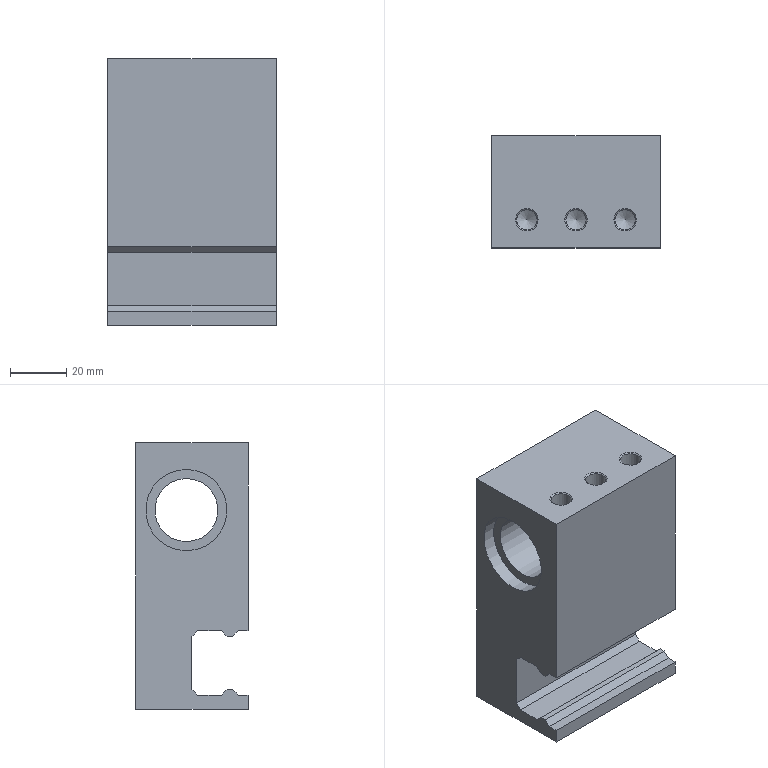Part | NX | features SIMPLE HOLE 8, SYMBOLIC_THREAD 7, DATUM_CSYS 5, HOLE PACKAGE 4, SKETCH 4, EXTRUDE 2, SUBTRACT 1 | 1 solid | 43 faces | box 60 x 40 x 95 mm | volume 172371 mm3 | plane 22 | cone 12 | cylinder 9 | commonest cylinder face diameters 5.2 x3 7.2 x3 29 x2 22.5 x1
STEP:
#1=CARTESIAN_POINT('',(-30.,-3.5,11.5));
#2=VERTEX_POINT('',#1);
#3=CARTESIAN_POINT('',(30.,-3.5,11.5));
#4=VERTEX_POINT('',#3);
#5=CARTESIAN_POINT('',(30.,-3.5,11.5));
#6=DIRECTION('',(-1.,0.,0.));
#7=VECTOR('',#6,1000.);
#8=LINE('',#5,#7);
#9=EDGE_CURVE('',#2,#4,#8,.F.);
#10=ORIENTED_EDGE('',*,*,#9,.T.);
#11=CARTESIAN_POINT('',(30.,-3.5,78.5));
#12=VERTEX_POINT('',#11);
#13=CARTESIAN_POINT('',(30.,-3.5,78.5));
#14=DIRECTION('',(0.,0.,-1.));
#15=VECTOR('',#14,1000.);
#16=LINE('',#13,#15);
#17=EDGE_CURVE('',#12,#4,#16,.T.);
#18=ORIENTED_EDGE('',*,*,#17,.F.);
#19=CARTESIAN_POINT('',(-30.,-3.5,78.5));
#20=VERTEX_POINT('',#19);
#21=CARTESIAN_POINT('',(30.,-3.5,78.5));
#22=DIRECTION('',(-1.,0.,0.));
#23=VECTOR('',#22,1000.);
#24=LINE('',#21,#23);
#25=EDGE_CURVE('',#12,#20,#24,.T.);
#26=ORIENTED_EDGE('',*,*,#25,.T.);
#27=CARTESIAN_POINT('',(-30.,-3.5,78.5));
#28=DIRECTION('',(0.,0.,-1.));
#29=VECTOR('',#28,1000.);
#30=LINE('',#27,#29);
#31=EDGE_CURVE('',#20,#2,#30,.T.);
#32=ORIENTED_EDGE('',*,*,#31,.T.);
#33=EDGE_LOOP('',(#10,#18,#26,#32));
#34=FACE_BOUND('',#33,.T.);
#35=CARTESIAN_POINT('',(30.,-3.5,78.5));
#36=DIRECTION('',(0.,1.,0.));
#37=DIRECTION('',(0.,0.,1.));
#38=AXIS2_PLACEMENT_3D('',#35,#36,#37);
#39=PLANE('',#38);
#40=ADVANCED_FACE('',(#34),#39,.F.);
#41=CARTESIAN_POINT('',(30.,-3.5,-11.5));
#42=VERTEX_POINT('',#41);
#43=CARTESIAN_POINT('',(-30.,-3.5,-11.5));
#44=VERTEX_POINT('',#43);
#45=CARTESIAN_POINT('',(30.,-3.5,-11.5));
#46=DIRECTION('',(1.,0.,0.));
#47=VECTOR('',#46,1000.);
#48=LINE('',#45,#47);
#49=EDGE_CURVE('',#42,#44,#48,.F.);
#50=ORIENTED_EDGE('',*,*,#49,.T.);
#51=CARTESIAN_POINT('',(-30.,-3.5,-16.5));
#52=VERTEX_POINT('',#51);
#53=CARTESIAN_POINT('',(-30.,-3.5,78.5));
#54=DIRECTION('',(0.,0.,-1.));
#55=VECTOR('',#54,1000.);
#56=LINE('',#53,#55);
#57=EDGE_CURVE('',#44,#52,#56,.T.);
#58=ORIENTED_EDGE('',*,*,#57,.T.);
#59=CARTESIAN_POINT('',(30.,-3.5,-16.5));
#60=VERTEX_POINT('',#59);
#61=CARTESIAN_POINT('',(30.,-3.5,-16.5));
#62=DIRECTION('',(-1.,0.,0.));
#63=VECTOR('',#62,1000.);
#64=LINE('',#61,#63);
#65=EDGE_CURVE('',#60,#52,#64,.T.);
#66=ORIENTED_EDGE('',*,*,#65,.F.);
#67=CARTESIAN_POINT('',(30.,-3.5,78.5));
#68=DIRECTION('',(0.,0.,-1.));
#69=VECTOR('',#68,1000.);
#70=LINE('',#67,#69);
#71=EDGE_CURVE('',#42,#60,#70,.T.);
#72=ORIENTED_EDGE('',*,*,#71,.F.);
#73=EDGE_LOOP('',(#50,#58,#66,#72));
#74=FACE_BOUND('',#73,.T.);
#75=CARTESIAN_POINT('',(30.,-3.5,78.5));
#76=DIRECTION('',(0.,1.,0.));
#77=DIRECTION('',(0.,0.,1.));
#78=AXIS2_PLACEMENT_3D('',#75,#76,#77);
#79=PLANE('',#78);
#80=ADVANCED_FACE('',(#74),#79,.F.);
#81=CARTESIAN_POINT('',(30.,18.5,69.));
#82=VERTEX_POINT('',#81);
#83=CARTESIAN_POINT('',(30.,18.5,54.5));
#84=DIRECTION('',(-1.,0.,0.));
#85=DIRECTION('',(0.,0.,1.));
#86=AXIS2_PLACEMENT_3D('',#83,#84,#85);
#87=CIRCLE('',#86,14.5);
#88=EDGE_CURVE('',#82,#82,#87,.T.);
#89=ORIENTED_EDGE('',*,*,#88,.T.);
#90=EDGE_LOOP('',(#89));
#91=FACE_BOUND('',#90,.T.);
#92=ORIENTED_EDGE('',*,*,#17,.T.);
#93=CARTESIAN_POINT('',(30.,0.,11.5));
#94=VERTEX_POINT('',#93);
#95=CARTESIAN_POINT('',(30.,18.5,11.5));
#96=DIRECTION('',(0.,1.,0.));
#97=VECTOR('',#96,1000.);
#98=LINE('',#95,#97);
#99=EDGE_CURVE('',#94,#4,#98,.F.);
#100=ORIENTED_EDGE('',*,*,#99,.F.);
#101=CARTESIAN_POINT('',(30.,2.,9.5));
#102=VERTEX_POINT('',#101);
#103=CARTESIAN_POINT('',(30.,-12.25,23.75));
#104=DIRECTION('',(0.,0.7071,-0.7071));
#105=VECTOR('',#104,1000.);
#106=LINE('',#103,#105);
#107=EDGE_CURVE('',#102,#94,#106,.F.);
#108=ORIENTED_EDGE('',*,*,#107,.F.);
#109=CARTESIAN_POINT('',(30.,4.,9.5));
#110=VERTEX_POINT('',#109);
#111=CARTESIAN_POINT('',(30.,18.5,9.5));
#112=DIRECTION('',(0.,1.,0.));
#113=VECTOR('',#112,1000.);
#114=LINE('',#111,#113);
#115=EDGE_CURVE('',#110,#102,#114,.F.);
#116=ORIENTED_EDGE('',*,*,#115,.F.);
#117=CARTESIAN_POINT('',(30.,6.,11.5));
#118=VERTEX_POINT('',#117);
#119=CARTESIAN_POINT('',(30.,33.75,39.25));
#120=DIRECTION('',(0.,0.7071,0.7071));
#121=VECTOR('',#120,1000.);
#122=LINE('',#119,#121);
#123=EDGE_CURVE('',#118,#110,#122,.F.);
#124=ORIENTED_EDGE('',*,*,#123,.F.);
#125=CARTESIAN_POINT('',(30.,14.5,11.5));
#126=VERTEX_POINT('',#125);
#127=CARTESIAN_POINT('',(30.,18.5,11.5));
#128=DIRECTION('',(0.,1.,0.));
#129=VECTOR('',#128,1000.);
#130=LINE('',#127,#129);
#131=EDGE_CURVE('',#126,#118,#130,.F.);
#132=ORIENTED_EDGE('',*,*,#131,.F.);
#133=CARTESIAN_POINT('',(30.,16.5,9.5));
#134=VERTEX_POINT('',#133);
#135=CARTESIAN_POINT('',(30.,-5.,31.));
#136=DIRECTION('',(0.,0.7071,-0.7071));
#137=VECTOR('',#136,1000.);
#138=LINE('',#135,#137);
#139=EDGE_CURVE('',#134,#126,#138,.F.);
#140=ORIENTED_EDGE('',*,*,#139,.F.);
#141=CARTESIAN_POINT('',(30.,16.5,-9.5));
#142=VERTEX_POINT('',#141);
#143=CARTESIAN_POINT('',(30.,16.5,54.5));
#144=DIRECTION('',(0.,0.,-1.));
#145=VECTOR('',#144,1000.);
#146=LINE('',#143,#145);
#147=EDGE_CURVE('',#142,#134,#146,.F.);
#148=ORIENTED_EDGE('',*,*,#147,.F.);
#149=CARTESIAN_POINT('',(30.,14.5,-11.5));
#150=VERTEX_POINT('',#149);
#151=CARTESIAN_POINT('',(30.,49.5,23.5));
#152=DIRECTION('',(0.,-0.7071,-0.7071));
#153=VECTOR('',#152,1000.);
#154=LINE('',#151,#153);
#155=EDGE_CURVE('',#150,#142,#154,.F.);
#156=ORIENTED_EDGE('',*,*,#155,.F.);
#157=CARTESIAN_POINT('',(30.,6.,-11.5));
#158=VERTEX_POINT('',#157);
#159=CARTESIAN_POINT('',(30.,18.5,-11.5));
#160=DIRECTION('',(0.,-1.,0.));
#161=VECTOR('',#160,1000.);
#162=LINE('',#159,#161);
#163=EDGE_CURVE('',#158,#150,#162,.F.);
#164=ORIENTED_EDGE('',*,*,#163,.F.);
#165=CARTESIAN_POINT('',(30.,4.,-9.5));
#166=VERTEX_POINT('',#165);
#167=CARTESIAN_POINT('',(30.,-20.75,15.25));
#168=DIRECTION('',(0.,-0.7071,0.7071));
#169=VECTOR('',#168,1000.);
#170=LINE('',#167,#169);
#171=EDGE_CURVE('',#166,#158,#170,.F.);
#172=ORIENTED_EDGE('',*,*,#171,.F.);
#173=CARTESIAN_POINT('',(30.,2.,-9.5));
#174=VERTEX_POINT('',#173);
#175=CARTESIAN_POINT('',(30.,18.5,-9.5));
#176=DIRECTION('',(0.,-1.,0.));
#177=VECTOR('',#176,1000.);
#178=LINE('',#175,#177);
#179=EDGE_CURVE('',#174,#166,#178,.F.);
#180=ORIENTED_EDGE('',*,*,#179,.F.);
#181=CARTESIAN_POINT('',(30.,0.,-11.5));
#182=VERTEX_POINT('',#181);
#183=CARTESIAN_POINT('',(30.,42.25,30.75));
#184=DIRECTION('',(0.,-0.7071,-0.7071));
#185=VECTOR('',#184,1000.);
#186=LINE('',#183,#185);
#187=EDGE_CURVE('',#182,#174,#186,.F.);
#188=ORIENTED_EDGE('',*,*,#187,.F.);
#189=CARTESIAN_POINT('',(30.,18.5,-11.5));
#190=DIRECTION('',(0.,-1.,0.));
#191=VECTOR('',#190,1000.);
#192=LINE('',#189,#191);
#193=EDGE_CURVE('',#42,#182,#192,.F.);
#194=ORIENTED_EDGE('',*,*,#193,.F.);
#195=ORIENTED_EDGE('',*,*,#71,.T.);
#196=CARTESIAN_POINT('',(30.,36.5,-16.5));
#197=VERTEX_POINT('',#196);
#198=CARTESIAN_POINT('',(30.,-3.5,-16.5));
#199=DIRECTION('',(0.,1.,0.));
#200=VECTOR('',#199,1000.);
#201=LINE('',#198,#200);
#202=EDGE_CURVE('',#60,#197,#201,.T.);
#203=ORIENTED_EDGE('',*,*,#202,.T.);
#204=CARTESIAN_POINT('',(30.,36.5,78.5));
#205=VERTEX_POINT('',#204);
#206=CARTESIAN_POINT('',(30.,36.5,-16.5));
#207=DIRECTION('',(0.,0.,1.));
#208=VECTOR('',#207,1000.);
#209=LINE('',#206,#208);
#210=EDGE_CURVE('',#197,#205,#209,.T.);
#211=ORIENTED_EDGE('',*,*,#210,.T.);
#212=CARTESIAN_POINT('',(30.,36.5,78.5));
#213=DIRECTION('',(0.,-1.,0.));
#214=VECTOR('',#213,1000.);
#215=LINE('',#212,#214);
#216=EDGE_CURVE('',#205,#12,#215,.T.);
#217=ORIENTED_EDGE('',*,*,#216,.T.);
#218=EDGE_LOOP('',(#92,#100,#108,#116,#124,#132,#140,#148,#156,#164,#172,#180,#188,#194,#195,#203,#211,#217));
#219=FACE_BOUND('',#218,.T.);
#220=CARTESIAN_POINT('',(30.,18.5,54.5));
#221=DIRECTION('',(1.,0.,0.));
#222=DIRECTION('',(0.,0.,-1.));
#223=AXIS2_PLACEMENT_3D('',#220,#221,#222);
#224=PLANE('',#223);
#225=ADVANCED_FACE('',(#91,#219),#224,.T.);
#226=CARTESIAN_POINT('',(-30.,18.5,40.));
#227=VERTEX_POINT('',#226);
#228=CARTESIAN_POINT('',(-30.,18.5,54.5));
#229=DIRECTION('',(1.,0.,0.));
#230=DIRECTION('',(0.,0.,-1.));
#231=AXIS2_PLACEMENT_3D('',#228,#229,#230);
#232=CIRCLE('',#231,14.5);
#233=EDGE_CURVE('',#227,#227,#232,.T.);
#234=ORIENTED_EDGE('',*,*,#233,.T.);
#235=EDGE_LOOP('',(#234));
#236=FACE_BOUND('',#235,.T.);
#237=CARTESIAN_POINT('',(-30.,0.,11.5));
#238=VERTEX_POINT('',#237);
#239=CARTESIAN_POINT('',(-30.,18.5,11.5));
#240=DIRECTION('',(0.,1.,0.));
#241=VECTOR('',#240,1000.);
#242=LINE('',#239,#241);
#243=EDGE_CURVE('',#238,#2,#242,.F.);
#244=ORIENTED_EDGE('',*,*,#243,.T.);
#245=ORIENTED_EDGE('',*,*,#31,.F.);
#246=CARTESIAN_POINT('',(-30.,36.5,78.5));
#247=VERTEX_POINT('',#246);
#248=CARTESIAN_POINT('',(-30.,36.5,78.5));
#249=DIRECTION('',(0.,-1.,0.));
#250=VECTOR('',#249,1000.);
#251=LINE('',#248,#250);
#252=EDGE_CURVE('',#247,#20,#251,.T.);
#253=ORIENTED_EDGE('',*,*,#252,.F.);
#254=CARTESIAN_POINT('',(-30.,36.5,-16.5));
#255=VERTEX_POINT('',#254);
#256=CARTESIAN_POINT('',(-30.,36.5,-16.5));
#257=DIRECTION('',(0.,0.,1.));
#258=VECTOR('',#257,1000.);
#259=LINE('',#256,#258);
#260=EDGE_CURVE('',#255,#247,#259,.T.);
#261=ORIENTED_EDGE('',*,*,#260,.F.);
#262=CARTESIAN_POINT('',(-30.,-3.5,-16.5));
#263=DIRECTION('',(0.,1.,0.));
#264=VECTOR('',#263,1000.);
#265=LINE('',#262,#264);
#266=EDGE_CURVE('',#52,#255,#265,.T.);
#267=ORIENTED_EDGE('',*,*,#266,.F.);
#268=ORIENTED_EDGE('',*,*,#57,.F.);
#269=CARTESIAN_POINT('',(-30.,0.,-11.5));
#270=VERTEX_POINT('',#269);
#271=CARTESIAN_POINT('',(-30.,18.5,-11.5));
#272=DIRECTION('',(0.,-1.,0.));
#273=VECTOR('',#272,1000.);
#274=LINE('',#271,#273);
#275=EDGE_CURVE('',#44,#270,#274,.F.);
#276=ORIENTED_EDGE('',*,*,#275,.T.);
#277=CARTESIAN_POINT('',(-30.,2.,-9.5));
#278=VERTEX_POINT('',#277);
#279=CARTESIAN_POINT('',(-30.,42.25,30.75));
#280=DIRECTION('',(0.,-0.7071,-0.7071));
#281=VECTOR('',#280,1000.);
#282=LINE('',#279,#281);
#283=EDGE_CURVE('',#270,#278,#282,.F.);
#284=ORIENTED_EDGE('',*,*,#283,.T.);
#285=CARTESIAN_POINT('',(-30.,4.,-9.5));
#286=VERTEX_POINT('',#285);
#287=CARTESIAN_POINT('',(-30.,18.5,-9.5));
#288=DIRECTION('',(0.,-1.,0.));
#289=VECTOR('',#288,1000.);
#290=LINE('',#287,#289);
#291=EDGE_CURVE('',#278,#286,#290,.F.);
#292=ORIENTED_EDGE('',*,*,#291,.T.);
#293=CARTESIAN_POINT('',(-30.,6.,-11.5));
#294=VERTEX_POINT('',#293);
#295=CARTESIAN_POINT('',(-30.,-20.75,15.25));
#296=DIRECTION('',(0.,-0.7071,0.7071));
#297=VECTOR('',#296,1000.);
#298=LINE('',#295,#297);
#299=EDGE_CURVE('',#286,#294,#298,.F.);
#300=ORIENTED_EDGE('',*,*,#299,.T.);
#301=CARTESIAN_POINT('',(-30.,14.5,-11.5));
#302=VERTEX_POINT('',#301);
#303=CARTESIAN_POINT('',(-30.,18.5,-11.5));
#304=DIRECTION('',(0.,-1.,0.));
#305=VECTOR('',#304,1000.);
#306=LINE('',#303,#305);
#307=EDGE_CURVE('',#294,#302,#306,.F.);
#308=ORIENTED_EDGE('',*,*,#307,.T.);
#309=CARTESIAN_POINT('',(-30.,16.5,-9.5));
#310=VERTEX_POINT('',#309);
#311=CARTESIAN_POINT('',(-30.,49.5,23.5));
#312=DIRECTION('',(0.,-0.7071,-0.7071));
#313=VECTOR('',#312,1000.);
#314=LINE('',#311,#313);
#315=EDGE_CURVE('',#302,#310,#314,.F.);
#316=ORIENTED_EDGE('',*,*,#315,.T.);
#317=CARTESIAN_POINT('',(-30.,16.5,9.5));
#318=VERTEX_POINT('',#317);
#319=CARTESIAN_POINT('',(-30.,16.5,54.5));
#320=DIRECTION('',(0.,0.,-1.));
#321=VECTOR('',#320,1000.);
#322=LINE('',#319,#321);
#323=EDGE_CURVE('',#310,#318,#322,.F.);
#324=ORIENTED_EDGE('',*,*,#323,.T.);
#325=CARTESIAN_POINT('',(-30.,14.5,11.5));
#326=VERTEX_POINT('',#325);
#327=CARTESIAN_POINT('',(-30.,-5.,31.));
#328=DIRECTION('',(0.,0.7071,-0.7071));
#329=VECTOR('',#328,1000.);
#330=LINE('',#327,#329);
#331=EDGE_CURVE('',#318,#326,#330,.F.);
#332=ORIENTED_EDGE('',*,*,#331,.T.);
#333=CARTESIAN_POINT('',(-30.,6.,11.5));
#334=VERTEX_POINT('',#333);
#335=CARTESIAN_POINT('',(-30.,18.5,11.5));
#336=DIRECTION('',(0.,1.,0.));
#337=VECTOR('',#336,1000.);
#338=LINE('',#335,#337);
#339=EDGE_CURVE('',#326,#334,#338,.F.);
#340=ORIENTED_EDGE('',*,*,#339,.T.);
#341=CARTESIAN_POINT('',(-30.,4.,9.5));
#342=VERTEX_POINT('',#341);
#343=CARTESIAN_POINT('',(-30.,33.75,39.25));
#344=DIRECTION('',(0.,0.7071,0.7071));
#345=VECTOR('',#344,1000.);
#346=LINE('',#343,#345);
#347=EDGE_CURVE('',#334,#342,#346,.F.);
#348=ORIENTED_EDGE('',*,*,#347,.T.);
#349=CARTESIAN_POINT('',(-30.,2.,9.5));
#350=VERTEX_POINT('',#349);
#351=CARTESIAN_POINT('',(-30.,18.5,9.5));
#352=DIRECTION('',(0.,1.,0.));
#353=VECTOR('',#352,1000.);
#354=LINE('',#351,#353);
#355=EDGE_CURVE('',#342,#350,#354,.F.);
#356=ORIENTED_EDGE('',*,*,#355,.T.);
#357=CARTESIAN_POINT('',(-30.,-12.25,23.75));
#358=DIRECTION('',(0.,0.7071,-0.7071));
#359=VECTOR('',#358,1000.);
#360=LINE('',#357,#359);
#361=EDGE_CURVE('',#350,#238,#360,.F.);
#362=ORIENTED_EDGE('',*,*,#361,.T.);
#363=EDGE_LOOP('',(#244,#245,#253,#261,#267,#268,#276,#284,#292,#300,#308,#316,#324,#332,#340,#348,#356,#362));
#364=FACE_BOUND('',#363,.T.);
#365=CARTESIAN_POINT('',(-30.,18.5,54.5));
#366=DIRECTION('',(1.,0.,0.));
#367=DIRECTION('',(0.,0.,-1.));
#368=AXIS2_PLACEMENT_3D('',#365,#366,#367);
#369=PLANE('',#368);
#370=ADVANCED_FACE('',(#236,#364),#369,.F.);
#371=CARTESIAN_POINT('',(-9.,26.5,-16.5));
#372=VERTEX_POINT('',#371);
#373=CARTESIAN_POINT('',(-12.,26.5,-16.5));
#374=DIRECTION('',(0.,0.,1.));
#375=DIRECTION('',(1.,0.,0.));
#376=AXIS2_PLACEMENT_3D('',#373,#374,#375);
#377=CIRCLE('',#376,3.);
#378=EDGE_CURVE('',#372,#372,#377,.T.);
#379=ORIENTED_EDGE('',*,*,#378,.T.);
#380=EDGE_LOOP('',(#379));
#381=FACE_BOUND('',#380,.T.);
#382=CARTESIAN_POINT('',(2.,26.5,-16.5));
#383=VERTEX_POINT('',#382);
#384=CARTESIAN_POINT('',(-1.,26.5,-16.5));
#385=DIRECTION('',(0.,0.,1.));
#386=DIRECTION('',(1.,0.,0.));
#387=AXIS2_PLACEMENT_3D('',#384,#385,#386);
#388=CIRCLE('',#387,3.);
#389=EDGE_CURVE('',#383,#383,#388,.T.);
#390=ORIENTED_EDGE('',*,*,#389,.T.);
#391=EDGE_LOOP('',(#390));
#392=FACE_BOUND('',#391,.T.);
#393=CARTESIAN_POINT('',(13.,26.5,-16.5));
#394=VERTEX_POINT('',#393);
#395=CARTESIAN_POINT('',(10.,26.5,-16.5));
#396=DIRECTION('',(0.,0.,1.));
#397=DIRECTION('',(1.,0.,0.));
#398=AXIS2_PLACEMENT_3D('',#395,#396,#397);
#399=CIRCLE('',#398,3.);
#400=EDGE_CURVE('',#394,#394,#399,.T.);
#401=ORIENTED_EDGE('',*,*,#400,.T.);
#402=EDGE_LOOP('',(#401));
#403=FACE_BOUND('',#402,.T.);
#404=ORIENTED_EDGE('',*,*,#266,.T.);
#405=CARTESIAN_POINT('',(30.,36.5,-16.5));
#406=DIRECTION('',(-1.,0.,0.));
#407=VECTOR('',#406,1000.);
#408=LINE('',#405,#407);
#409=EDGE_CURVE('',#197,#255,#408,.T.);
#410=ORIENTED_EDGE('',*,*,#409,.F.);
#411=ORIENTED_EDGE('',*,*,#202,.F.);
#412=ORIENTED_EDGE('',*,*,#65,.T.);
#413=EDGE_LOOP('',(#404,#410,#411,#412));
#414=FACE_BOUND('',#413,.T.);
#415=CARTESIAN_POINT('',(30.,-3.5,-16.5));
#416=DIRECTION('',(0.,0.,1.));
#417=DIRECTION('',(1.,0.,0.));
#418=AXIS2_PLACEMENT_3D('',#415,#416,#417);
#419=PLANE('',#418);
#420=ADVANCED_FACE('',(#381,#392,#403,#414),#419,.F.);
#421=ORIENTED_EDGE('',*,*,#260,.T.);
#422=CARTESIAN_POINT('',(30.,36.5,78.5));
#423=DIRECTION('',(-1.,0.,0.));
#424=VECTOR('',#423,1000.);
#425=LINE('',#422,#424);
#426=EDGE_CURVE('',#205,#247,#425,.T.);
#427=ORIENTED_EDGE('',*,*,#426,.F.);
#428=ORIENTED_EDGE('',*,*,#210,.F.);
#429=ORIENTED_EDGE('',*,*,#409,.T.);
#430=EDGE_LOOP('',(#421,#427,#428,#429));
#431=FACE_BOUND('',#430,.T.);
#432=CARTESIAN_POINT('',(30.,36.5,-16.5));
#433=DIRECTION('',(0.,-1.,0.));
#434=DIRECTION('',(0.,0.,-1.));
#435=AXIS2_PLACEMENT_3D('',#432,#433,#434);
#436=PLANE('',#435);
#437=ADVANCED_FACE('',(#431),#436,.F.);
#438=CARTESIAN_POINT('',(13.5,6.5,78.5));
#439=VERTEX_POINT('',#438);
#440=CARTESIAN_POINT('',(17.5,6.5,78.5));
#441=DIRECTION('',(0.,0.,-1.));
#442=DIRECTION('',(-1.,0.,0.));
#443=AXIS2_PLACEMENT_3D('',#440,#441,#442);
#444=CIRCLE('',#443,4.);
#445=EDGE_CURVE('',#439,#439,#444,.T.);
#446=ORIENTED_EDGE('',*,*,#445,.T.);
#447=EDGE_LOOP('',(#446));
#448=FACE_BOUND('',#447,.T.);
#449=CARTESIAN_POINT('',(-4.,6.5,78.5));
#450=VERTEX_POINT('',#449);
#451=CARTESIAN_POINT('',(0.,6.5,78.5));
#452=DIRECTION('',(0.,0.,-1.));
#453=DIRECTION('',(-1.,0.,0.));
#454=AXIS2_PLACEMENT_3D('',#451,#452,#453);
#455=CIRCLE('',#454,4.);
#456=EDGE_CURVE('',#450,#450,#455,.T.);
#457=ORIENTED_EDGE('',*,*,#456,.T.);
#458=EDGE_LOOP('',(#457));
#459=FACE_BOUND('',#458,.T.);
#460=CARTESIAN_POINT('',(-21.5,6.5,78.5));
#461=VERTEX_POINT('',#460);
#462=CARTESIAN_POINT('',(-17.5,6.5,78.5));
#463=DIRECTION('',(0.,0.,-1.));
#464=DIRECTION('',(-1.,0.,0.));
#465=AXIS2_PLACEMENT_3D('',#462,#463,#464);
#466=CIRCLE('',#465,4.);
#467=EDGE_CURVE('',#461,#461,#466,.T.);
#468=ORIENTED_EDGE('',*,*,#467,.T.);
#469=EDGE_LOOP('',(#468));
#470=FACE_BOUND('',#469,.T.);
#471=ORIENTED_EDGE('',*,*,#252,.T.);
#472=ORIENTED_EDGE('',*,*,#25,.F.);
#473=ORIENTED_EDGE('',*,*,#216,.F.);
#474=ORIENTED_EDGE('',*,*,#426,.T.);
#475=EDGE_LOOP('',(#471,#472,#473,#474));
#476=FACE_BOUND('',#475,.T.);
#477=CARTESIAN_POINT('',(30.,36.5,78.5));
#478=DIRECTION('',(0.,0.,-1.));
#479=DIRECTION('',(-1.,0.,0.));
#480=AXIS2_PLACEMENT_3D('',#477,#478,#479);
#481=PLANE('',#480);
#482=ADVANCED_FACE('',(#448,#459,#470,#476),#481,.F.);
#483=CARTESIAN_POINT('',(25.,18.5,65.75));
#484=VERTEX_POINT('',#483);
#485=CARTESIAN_POINT('',(25.,18.5,54.5));
#486=DIRECTION('',(-1.,0.,0.));
#487=DIRECTION('',(0.,0.,1.));
#488=AXIS2_PLACEMENT_3D('',#485,#486,#487);
#489=CIRCLE('',#488,11.25);
#490=EDGE_CURVE('',#484,#484,#489,.T.);
#491=ORIENTED_EDGE('',*,*,#490,.F.);
#492=EDGE_LOOP('',(#491));
#493=FACE_BOUND('',#492,.T.);
#494=CARTESIAN_POINT('',(-25.,18.5,43.25));
#495=VERTEX_POINT('',#494);
#496=CARTESIAN_POINT('',(-25.,18.5,54.5));
#497=DIRECTION('',(1.,0.,0.));
#498=DIRECTION('',(0.,0.,-1.));
#499=AXIS2_PLACEMENT_3D('',#496,#497,#498);
#500=CIRCLE('',#499,11.25);
#501=EDGE_CURVE('',#495,#495,#500,.T.);
#502=ORIENTED_EDGE('',*,*,#501,.F.);
#503=EDGE_LOOP('',(#502));
#504=FACE_BOUND('',#503,.T.);
#505=CARTESIAN_POINT('',(30.,18.5,54.5));
#506=DIRECTION('',(-1.,0.,0.));
#507=DIRECTION('',(0.,0.,1.));
#508=AXIS2_PLACEMENT_3D('',#505,#506,#507);
#509=CYLINDRICAL_SURFACE('',#508,11.25);
#510=ADVANCED_FACE('',(#493,#504),#509,.F.);
#511=CARTESIAN_POINT('',(225.,2.,-9.5));
#512=DIRECTION('',(-1.,0.,0.));
#513=VECTOR('',#512,1000.);
#514=LINE('',#511,#513);
#515=EDGE_CURVE('',#278,#174,#514,.F.);
#516=ORIENTED_EDGE('',*,*,#515,.F.);
#517=ORIENTED_EDGE('',*,*,#283,.F.);
#518=CARTESIAN_POINT('',(225.,0.,-11.5));
#519=DIRECTION('',(-1.,0.,0.));
#520=VECTOR('',#519,1000.);
#521=LINE('',#518,#520);
#522=EDGE_CURVE('',#270,#182,#521,.F.);
#523=ORIENTED_EDGE('',*,*,#522,.T.);
#524=ORIENTED_EDGE('',*,*,#187,.T.);
#525=EDGE_LOOP('',(#516,#517,#523,#524));
#526=FACE_BOUND('',#525,.T.);
#527=CARTESIAN_POINT('',(225.,0.,-11.5));
#528=DIRECTION('',(0.,-0.7071,0.7071));
#529=DIRECTION('',(0.,-0.7071,-0.7071));
#530=AXIS2_PLACEMENT_3D('',#527,#528,#529);
#531=PLANE('',#530);
#532=ADVANCED_FACE('',(#526),#531,.T.);
#533=CARTESIAN_POINT('',(225.,4.,-9.5));
#534=DIRECTION('',(-1.,0.,0.));
#535=VECTOR('',#534,1000.);
#536=LINE('',#533,#535);
#537=EDGE_CURVE('',#286,#166,#536,.F.);
#538=ORIENTED_EDGE('',*,*,#537,.F.);
#539=ORIENTED_EDGE('',*,*,#291,.F.);
#540=ORIENTED_EDGE('',*,*,#515,.T.);
#541=ORIENTED_EDGE('',*,*,#179,.T.);
#542=EDGE_LOOP('',(#538,#539,#540,#541));
#543=FACE_BOUND('',#542,.T.);
#544=CARTESIAN_POINT('',(225.,2.,-9.5));
#545=DIRECTION('',(0.,0.,1.));
#546=DIRECTION('',(1.,0.,0.));
#547=AXIS2_PLACEMENT_3D('',#544,#545,#546);
#548=PLANE('',#547);
#549=ADVANCED_FACE('',(#543),#548,.T.);
#550=CARTESIAN_POINT('',(225.,6.,-11.5));
#551=DIRECTION('',(-1.,0.,0.));
#552=VECTOR('',#551,1000.);
#553=LINE('',#550,#552);
#554=EDGE_CURVE('',#294,#158,#553,.F.);
#555=ORIENTED_EDGE('',*,*,#554,.F.);
#556=ORIENTED_EDGE('',*,*,#299,.F.);
#557=ORIENTED_EDGE('',*,*,#537,.T.);
#558=ORIENTED_EDGE('',*,*,#171,.T.);
#559=EDGE_LOOP('',(#555,#556,#557,#558));
#560=FACE_BOUND('',#559,.T.);
#561=CARTESIAN_POINT('',(225.,4.,-9.5));
#562=DIRECTION('',(0.,0.7071,0.7071));
#563=DIRECTION('',(0.,-0.7071,0.7071));
#564=AXIS2_PLACEMENT_3D('',#561,#562,#563);
#565=PLANE('',#564);
#566=ADVANCED_FACE('',(#560),#565,.T.);
#567=CARTESIAN_POINT('',(225.,14.5,-11.5));
#568=DIRECTION('',(-1.,0.,0.));
#569=VECTOR('',#568,1000.);
#570=LINE('',#567,#569);
#571=EDGE_CURVE('',#302,#150,#570,.F.);
#572=ORIENTED_EDGE('',*,*,#571,.F.);
#573=ORIENTED_EDGE('',*,*,#307,.F.);
#574=ORIENTED_EDGE('',*,*,#554,.T.);
#575=ORIENTED_EDGE('',*,*,#163,.T.);
#576=EDGE_LOOP('',(#572,#573,#574,#575));
#577=FACE_BOUND('',#576,.T.);
#578=CARTESIAN_POINT('',(225.,6.,-11.5));
#579=DIRECTION('',(0.,0.,1.));
#580=DIRECTION('',(0.,-1.,0.));
#581=AXIS2_PLACEMENT_3D('',#578,#579,#580);
#582=PLANE('',#581);
#583=ADVANCED_FACE('',(#577),#582,.T.);
#584=CARTESIAN_POINT('',(225.,16.5,-9.5));
#585=DIRECTION('',(-1.,0.,0.));
#586=VECTOR('',#585,1000.);
#587=LINE('',#584,#586);
#588=EDGE_CURVE('',#310,#142,#587,.F.);
#589=ORIENTED_EDGE('',*,*,#588,.F.);
#590=ORIENTED_EDGE('',*,*,#315,.F.);
#591=ORIENTED_EDGE('',*,*,#571,.T.);
#592=ORIENTED_EDGE('',*,*,#155,.T.);
#593=EDGE_LOOP('',(#589,#590,#591,#592));
#594=FACE_BOUND('',#593,.T.);
#595=CARTESIAN_POINT('',(225.,14.5,-11.5));
#596=DIRECTION('',(0.,-0.7071,0.7071));
#597=DIRECTION('',(0.,-0.7071,-0.7071));
#598=AXIS2_PLACEMENT_3D('',#595,#596,#597);
#599=PLANE('',#598);
#600=ADVANCED_FACE('',(#594),#599,.T.);
#601=CARTESIAN_POINT('',(225.,16.5,9.5));
#602=DIRECTION('',(-1.,0.,0.));
#603=VECTOR('',#602,1000.);
#604=LINE('',#601,#603);
#605=EDGE_CURVE('',#318,#134,#604,.F.);
#606=ORIENTED_EDGE('',*,*,#605,.F.);
#607=ORIENTED_EDGE('',*,*,#323,.F.);
#608=ORIENTED_EDGE('',*,*,#588,.T.);
#609=ORIENTED_EDGE('',*,*,#147,.T.);
#610=EDGE_LOOP('',(#606,#607,#608,#609));
#611=FACE_BOUND('',#610,.T.);
#612=CARTESIAN_POINT('',(225.,16.5,0.));
#613=DIRECTION('',(0.,-1.,0.));
#614=DIRECTION('',(0.,0.,-1.));
#615=AXIS2_PLACEMENT_3D('',#612,#613,#614);
#616=PLANE('',#615);
#617=ADVANCED_FACE('',(#611),#616,.T.);
#618=CARTESIAN_POINT('',(225.,14.5,11.5));
#619=DIRECTION('',(-1.,0.,0.));
#620=VECTOR('',#619,1000.);
#621=LINE('',#618,#620);
#622=EDGE_CURVE('',#326,#126,#621,.F.);
#623=ORIENTED_EDGE('',*,*,#622,.F.);
#624=ORIENTED_EDGE('',*,*,#331,.F.);
#625=ORIENTED_EDGE('',*,*,#605,.T.);
#626=ORIENTED_EDGE('',*,*,#139,.T.);
#627=EDGE_LOOP('',(#623,#624,#625,#626));
#628=FACE_BOUND('',#627,.T.);
#629=CARTESIAN_POINT('',(225.,16.5,9.5));
#630=DIRECTION('',(0.,-0.7071,-0.7071));
#631=DIRECTION('',(0.,0.7071,-0.7071));
#632=AXIS2_PLACEMENT_3D('',#629,#630,#631);
#633=PLANE('',#632);
#634=ADVANCED_FACE('',(#628),#633,.T.);
#635=CARTESIAN_POINT('',(225.,6.,11.5));
#636=DIRECTION('',(-1.,0.,0.));
#637=VECTOR('',#636,1000.);
#638=LINE('',#635,#637);
#639=EDGE_CURVE('',#334,#118,#638,.F.);
#640=ORIENTED_EDGE('',*,*,#639,.F.);
#641=ORIENTED_EDGE('',*,*,#339,.F.);
#642=ORIENTED_EDGE('',*,*,#622,.T.);
#643=ORIENTED_EDGE('',*,*,#131,.T.);
#644=EDGE_LOOP('',(#640,#641,#642,#643));
#645=FACE_BOUND('',#644,.T.);
#646=CARTESIAN_POINT('',(225.,14.5,11.5));
#647=DIRECTION('',(0.,0.,-1.));
#648=DIRECTION('',(0.,1.,0.));
#649=AXIS2_PLACEMENT_3D('',#646,#647,#648);
#650=PLANE('',#649);
#651=ADVANCED_FACE('',(#645),#650,.T.);
#652=CARTESIAN_POINT('',(225.,4.,9.5));
#653=DIRECTION('',(-1.,0.,0.));
#654=VECTOR('',#653,1000.);
#655=LINE('',#652,#654);
#656=EDGE_CURVE('',#342,#110,#655,.F.);
#657=ORIENTED_EDGE('',*,*,#656,.F.);
#658=ORIENTED_EDGE('',*,*,#347,.F.);
#659=ORIENTED_EDGE('',*,*,#639,.T.);
#660=ORIENTED_EDGE('',*,*,#123,.T.);
#661=EDGE_LOOP('',(#657,#658,#659,#660));
#662=FACE_BOUND('',#661,.T.);
#663=CARTESIAN_POINT('',(225.,6.,11.5));
#664=DIRECTION('',(0.,0.7071,-0.7071));
#665=DIRECTION('',(0.,0.7071,0.7071));
#666=AXIS2_PLACEMENT_3D('',#663,#664,#665);
#667=PLANE('',#666);
#668=ADVANCED_FACE('',(#662),#667,.T.);
#669=CARTESIAN_POINT('',(225.,2.,9.5));
#670=DIRECTION('',(-1.,0.,0.));
#671=VECTOR('',#670,1000.);
#672=LINE('',#669,#671);
#673=EDGE_CURVE('',#350,#102,#672,.F.);
#674=ORIENTED_EDGE('',*,*,#673,.F.);
#675=ORIENTED_EDGE('',*,*,#355,.F.);
#676=ORIENTED_EDGE('',*,*,#656,.T.);
#677=ORIENTED_EDGE('',*,*,#115,.T.);
#678=EDGE_LOOP('',(#674,#675,#676,#677));
#679=FACE_BOUND('',#678,.T.);
#680=CARTESIAN_POINT('',(225.,4.,9.5));
#681=DIRECTION('',(0.,0.,-1.));
#682=DIRECTION('',(-1.,0.,0.));
#683=AXIS2_PLACEMENT_3D('',#680,#681,#682);
#684=PLANE('',#683);
#685=ADVANCED_FACE('',(#679),#684,.T.);
#686=CARTESIAN_POINT('',(225.,0.,11.5));
#687=DIRECTION('',(-1.,0.,0.));
#688=VECTOR('',#687,1000.);
#689=LINE('',#686,#688);
#690=EDGE_CURVE('',#238,#94,#689,.F.);
#691=ORIENTED_EDGE('',*,*,#690,.F.);
#692=ORIENTED_EDGE('',*,*,#361,.F.);
#693=ORIENTED_EDGE('',*,*,#673,.T.);
#694=ORIENTED_EDGE('',*,*,#107,.T.);
#695=EDGE_LOOP('',(#691,#692,#693,#694));
#696=FACE_BOUND('',#695,.T.);
#697=CARTESIAN_POINT('',(225.,2.,9.5));
#698=DIRECTION('',(0.,-0.7071,-0.7071));
#699=DIRECTION('',(0.,0.7071,-0.7071));
#700=AXIS2_PLACEMENT_3D('',#697,#698,#699);
#701=PLANE('',#700);
#702=ADVANCED_FACE('',(#696),#701,.T.);
#703=ORIENTED_EDGE('',*,*,#9,.F.);
#704=ORIENTED_EDGE('',*,*,#243,.F.);
#705=ORIENTED_EDGE('',*,*,#690,.T.);
#706=ORIENTED_EDGE('',*,*,#99,.T.);
#707=EDGE_LOOP('',(#703,#704,#705,#706));
#708=FACE_BOUND('',#707,.T.);
#709=CARTESIAN_POINT('',(225.,0.,11.5));
#710=DIRECTION('',(0.,0.,-1.));
#711=DIRECTION('',(0.,1.,0.));
#712=AXIS2_PLACEMENT_3D('',#709,#710,#711);
#713=PLANE('',#712);
#714=ADVANCED_FACE('',(#708),#713,.T.);
#715=ORIENTED_EDGE('',*,*,#522,.F.);
#716=ORIENTED_EDGE('',*,*,#275,.F.);
#717=ORIENTED_EDGE('',*,*,#49,.F.);
#718=ORIENTED_EDGE('',*,*,#193,.T.);
#719=EDGE_LOOP('',(#715,#716,#717,#718));
#720=FACE_BOUND('',#719,.T.);
#721=CARTESIAN_POINT('',(225.,-5.5,-11.5));
#722=DIRECTION('',(0.,0.,1.));
#723=DIRECTION('',(0.,-1.,0.));
#724=AXIS2_PLACEMENT_3D('',#721,#722,#723);
#725=PLANE('',#724);
#726=ADVANCED_FACE('',(#720),#725,.T.);
#727=CARTESIAN_POINT('',(12.6,26.5,1.5));
#728=VERTEX_POINT('',#727);
#729=CARTESIAN_POINT('',(10.,26.5,1.5));
#730=DIRECTION('',(0.,0.,1.));
#731=DIRECTION('',(1.,0.,0.));
#732=AXIS2_PLACEMENT_3D('',#729,#730,#731);
#733=CIRCLE('',#732,2.6);
#734=EDGE_CURVE('',#728,#728,#733,.F.);
#735=ORIENTED_EDGE('',*,*,#734,.T.);
#736=EDGE_LOOP('',(#735));
#737=FACE_BOUND('',#736,.T.);
#738=CARTESIAN_POINT('',(10.,26.5,3.062));
#739=VERTEX_POINT('',#738);
#740=VERTEX_LOOP('',#739);
#741=FACE_BOUND('',#740,.T.);
#742=CARTESIAN_POINT('',(10.,26.5,1.5));
#743=DIRECTION('',(0.,0.,-1.));
#744=DIRECTION('',(-1.,0.,0.));
#745=AXIS2_PLACEMENT_3D('',#742,#743,#744);
#746=CONICAL_SURFACE('',#745,2.6,1.03);
#747=ADVANCED_FACE('',(#737,#741),#746,.F.);
#748=CARTESIAN_POINT('',(12.6,26.5,-16.1));
#749=VERTEX_POINT('',#748);
#750=CARTESIAN_POINT('',(10.,26.5,-16.1));
#751=DIRECTION('',(0.,0.,1.));
#752=DIRECTION('',(1.,0.,0.));
#753=AXIS2_PLACEMENT_3D('',#750,#751,#752);
#754=CIRCLE('',#753,2.6);
#755=EDGE_CURVE('',#749,#749,#754,.F.);
#756=ORIENTED_EDGE('',*,*,#755,.T.);
#757=EDGE_LOOP('',(#756));
#758=FACE_BOUND('',#757,.T.);
#759=ORIENTED_EDGE('',*,*,#734,.F.);
#760=EDGE_LOOP('',(#759));
#761=FACE_BOUND('',#760,.T.);
#762=CARTESIAN_POINT('',(10.,26.5,-16.5));
#763=DIRECTION('',(0.,0.,1.));
#764=DIRECTION('',(1.,0.,0.));
#765=AXIS2_PLACEMENT_3D('',#762,#763,#764);
#766=CYLINDRICAL_SURFACE('',#765,2.6);
#767=ADVANCED_FACE('',(#758,#761),#766,.F.);
#768=ORIENTED_EDGE('',*,*,#755,.F.);
#769=EDGE_LOOP('',(#768));
#770=FACE_BOUND('',#769,.T.);
#771=ORIENTED_EDGE('',*,*,#400,.F.);
#772=EDGE_LOOP('',(#771));
#773=FACE_BOUND('',#772,.T.);
#774=CARTESIAN_POINT('',(10.,26.5,-16.5));
#775=DIRECTION('',(0.,0.,-1.));
#776=DIRECTION('',(-1.,0.,0.));
#777=AXIS2_PLACEMENT_3D('',#774,#775,#776);
#778=CONICAL_SURFACE('',#777,3.,0.7854);
#779=ADVANCED_FACE('',(#770,#773),#778,.F.);
#780=CARTESIAN_POINT('',(1.6,26.5,1.5));
#781=VERTEX_POINT('',#780);
#782=CARTESIAN_POINT('',(-1.,26.5,1.5));
#783=DIRECTION('',(0.,0.,1.));
#784=DIRECTION('',(1.,0.,0.));
#785=AXIS2_PLACEMENT_3D('',#782,#783,#784);
#786=CIRCLE('',#785,2.6);
#787=EDGE_CURVE('',#781,#781,#786,.F.);
#788=ORIENTED_EDGE('',*,*,#787,.T.);
#789=EDGE_LOOP('',(#788));
#790=FACE_BOUND('',#789,.T.);
#791=CARTESIAN_POINT('',(-1.,26.5,3.062));
#792=VERTEX_POINT('',#791);
#793=VERTEX_LOOP('',#792);
#794=FACE_BOUND('',#793,.T.);
#795=CARTESIAN_POINT('',(-1.,26.5,1.5));
#796=DIRECTION('',(0.,0.,-1.));
#797=DIRECTION('',(-1.,0.,0.));
#798=AXIS2_PLACEMENT_3D('',#795,#796,#797);
#799=CONICAL_SURFACE('',#798,2.6,1.03);
#800=ADVANCED_FACE('',(#790,#794),#799,.F.);
#801=CARTESIAN_POINT('',(1.6,26.5,-16.1));
#802=VERTEX_POINT('',#801);
#803=CARTESIAN_POINT('',(-1.,26.5,-16.1));
#804=DIRECTION('',(0.,0.,1.));
#805=DIRECTION('',(1.,0.,0.));
#806=AXIS2_PLACEMENT_3D('',#803,#804,#805);
#807=CIRCLE('',#806,2.6);
#808=EDGE_CURVE('',#802,#802,#807,.F.);
#809=ORIENTED_EDGE('',*,*,#808,.T.);
#810=EDGE_LOOP('',(#809));
#811=FACE_BOUND('',#810,.T.);
#812=ORIENTED_EDGE('',*,*,#787,.F.);
#813=EDGE_LOOP('',(#812));
#814=FACE_BOUND('',#813,.T.);
#815=CARTESIAN_POINT('',(-1.,26.5,-16.5));
#816=DIRECTION('',(0.,0.,1.));
#817=DIRECTION('',(1.,0.,0.));
#818=AXIS2_PLACEMENT_3D('',#815,#816,#817);
#819=CYLINDRICAL_SURFACE('',#818,2.6);
#820=ADVANCED_FACE('',(#811,#814),#819,.F.);
#821=ORIENTED_EDGE('',*,*,#808,.F.);
#822=EDGE_LOOP('',(#821));
#823=FACE_BOUND('',#822,.T.);
#824=ORIENTED_EDGE('',*,*,#389,.F.);
#825=EDGE_LOOP('',(#824));
#826=FACE_BOUND('',#825,.T.);
#827=CARTESIAN_POINT('',(-1.,26.5,-16.5));
#828=DIRECTION('',(0.,0.,-1.));
#829=DIRECTION('',(-1.,0.,0.));
#830=AXIS2_PLACEMENT_3D('',#827,#828,#829);
#831=CONICAL_SURFACE('',#830,3.,0.7854);
#832=ADVANCED_FACE('',(#823,#826),#831,.F.);
#833=CARTESIAN_POINT('',(-9.4,26.5,1.5));
#834=VERTEX_POINT('',#833);
#835=CARTESIAN_POINT('',(-12.,26.5,1.5));
#836=DIRECTION('',(0.,0.,1.));
#837=DIRECTION('',(1.,0.,0.));
#838=AXIS2_PLACEMENT_3D('',#835,#836,#837);
#839=CIRCLE('',#838,2.6);
#840=EDGE_CURVE('',#834,#834,#839,.F.);
#841=ORIENTED_EDGE('',*,*,#840,.T.);
#842=EDGE_LOOP('',(#841));
#843=FACE_BOUND('',#842,.T.);
#844=CARTESIAN_POINT('',(-12.,26.5,3.062));
#845=VERTEX_POINT('',#844);
#846=VERTEX_LOOP('',#845);
#847=FACE_BOUND('',#846,.T.);
#848=CARTESIAN_POINT('',(-12.,26.5,1.5));
#849=DIRECTION('',(0.,0.,-1.));
#850=DIRECTION('',(-1.,0.,0.));
#851=AXIS2_PLACEMENT_3D('',#848,#849,#850);
#852=CONICAL_SURFACE('',#851,2.6,1.03);
#853=ADVANCED_FACE('',(#843,#847),#852,.F.);
#854=CARTESIAN_POINT('',(-9.4,26.5,-16.1));
#855=VERTEX_POINT('',#854);
#856=CARTESIAN_POINT('',(-12.,26.5,-16.1));
#857=DIRECTION('',(0.,0.,1.));
#858=DIRECTION('',(1.,0.,0.));
#859=AXIS2_PLACEMENT_3D('',#856,#857,#858);
#860=CIRCLE('',#859,2.6);
#861=EDGE_CURVE('',#855,#855,#860,.F.);
#862=ORIENTED_EDGE('',*,*,#861,.T.);
#863=EDGE_LOOP('',(#862));
#864=FACE_BOUND('',#863,.T.);
#865=ORIENTED_EDGE('',*,*,#840,.F.);
#866=EDGE_LOOP('',(#865));
#867=FACE_BOUND('',#866,.T.);
#868=CARTESIAN_POINT('',(-12.,26.5,-16.5));
#869=DIRECTION('',(0.,0.,1.));
#870=DIRECTION('',(1.,0.,0.));
#871=AXIS2_PLACEMENT_3D('',#868,#869,#870);
#872=CYLINDRICAL_SURFACE('',#871,2.6);
#873=ADVANCED_FACE('',(#864,#867),#872,.F.);
#874=ORIENTED_EDGE('',*,*,#861,.F.);
#875=EDGE_LOOP('',(#874));
#876=FACE_BOUND('',#875,.T.);
#877=ORIENTED_EDGE('',*,*,#378,.F.);
#878=EDGE_LOOP('',(#877));
#879=FACE_BOUND('',#878,.T.);
#880=CARTESIAN_POINT('',(-12.,26.5,-16.5));
#881=DIRECTION('',(0.,0.,-1.));
#882=DIRECTION('',(-1.,0.,0.));
#883=AXIS2_PLACEMENT_3D('',#880,#881,#882);
#884=CONICAL_SURFACE('',#883,3.,0.7854);
#885=ADVANCED_FACE('',(#876,#879),#884,.F.);
#886=CARTESIAN_POINT('',(-21.1,6.5,66.5));
#887=VERTEX_POINT('',#886);
#888=CARTESIAN_POINT('',(-17.5,6.5,66.5));
#889=DIRECTION('',(0.,0.,-1.));
#890=DIRECTION('',(-1.,0.,0.));
#891=AXIS2_PLACEMENT_3D('',#888,#889,#890);
#892=CIRCLE('',#891,3.6);
#893=EDGE_CURVE('',#887,#887,#892,.F.);
#894=ORIENTED_EDGE('',*,*,#893,.T.);
#895=EDGE_LOOP('',(#894));
#896=FACE_BOUND('',#895,.T.);
#897=CARTESIAN_POINT('',(-17.5,6.5,64.337));
#898=VERTEX_POINT('',#897);
#899=VERTEX_LOOP('',#898);
#900=FACE_BOUND('',#899,.T.);
#901=CARTESIAN_POINT('',(-17.5,6.5,66.5));
#902=DIRECTION('',(0.,0.,1.));
#903=DIRECTION('',(1.,0.,0.));
#904=AXIS2_PLACEMENT_3D('',#901,#902,#903);
#905=CONICAL_SURFACE('',#904,3.6,1.03);
#906=ADVANCED_FACE('',(#896,#900),#905,.F.);
#907=CARTESIAN_POINT('',(-21.1,6.5,78.1));
#908=VERTEX_POINT('',#907);
#909=CARTESIAN_POINT('',(-17.5,6.5,78.1));
#910=DIRECTION('',(0.,0.,-1.));
#911=DIRECTION('',(-1.,0.,0.));
#912=AXIS2_PLACEMENT_3D('',#909,#910,#911);
#913=CIRCLE('',#912,3.6);
#914=EDGE_CURVE('',#908,#908,#913,.F.);
#915=ORIENTED_EDGE('',*,*,#914,.T.);
#916=EDGE_LOOP('',(#915));
#917=FACE_BOUND('',#916,.T.);
#918=ORIENTED_EDGE('',*,*,#893,.F.);
#919=EDGE_LOOP('',(#918));
#920=FACE_BOUND('',#919,.T.);
#921=CARTESIAN_POINT('',(-17.5,6.5,78.5));
#922=DIRECTION('',(0.,0.,-1.));
#923=DIRECTION('',(-1.,0.,0.));
#924=AXIS2_PLACEMENT_3D('',#921,#922,#923);
#925=CYLINDRICAL_SURFACE('',#924,3.6);
#926=ADVANCED_FACE('',(#917,#920),#925,.F.);
#927=ORIENTED_EDGE('',*,*,#914,.F.);
#928=EDGE_LOOP('',(#927));
#929=FACE_BOUND('',#928,.T.);
#930=ORIENTED_EDGE('',*,*,#467,.F.);
#931=EDGE_LOOP('',(#930));
#932=FACE_BOUND('',#931,.T.);
#933=CARTESIAN_POINT('',(-17.5,6.5,78.5));
#934=DIRECTION('',(0.,0.,1.));
#935=DIRECTION('',(1.,0.,0.));
#936=AXIS2_PLACEMENT_3D('',#933,#934,#935);
#937=CONICAL_SURFACE('',#936,4.,0.7854);
#938=ADVANCED_FACE('',(#929,#932),#937,.F.);
#939=CARTESIAN_POINT('',(-3.6,6.5,66.5));
#940=VERTEX_POINT('',#939);
#941=CARTESIAN_POINT('',(0.,6.5,66.5));
#942=DIRECTION('',(0.,0.,-1.));
#943=DIRECTION('',(-1.,0.,0.));
#944=AXIS2_PLACEMENT_3D('',#941,#942,#943);
#945=CIRCLE('',#944,3.6);
#946=EDGE_CURVE('',#940,#940,#945,.F.);
#947=ORIENTED_EDGE('',*,*,#946,.T.);
#948=EDGE_LOOP('',(#947));
#949=FACE_BOUND('',#948,.T.);
#950=CARTESIAN_POINT('',(0.,6.5,64.337));
#951=VERTEX_POINT('',#950);
#952=VERTEX_LOOP('',#951);
#953=FACE_BOUND('',#952,.T.);
#954=CARTESIAN_POINT('',(0.,6.5,66.5));
#955=DIRECTION('',(0.,0.,1.));
#956=DIRECTION('',(1.,0.,0.));
#957=AXIS2_PLACEMENT_3D('',#954,#955,#956);
#958=CONICAL_SURFACE('',#957,3.6,1.03);
#959=ADVANCED_FACE('',(#949,#953),#958,.F.);
#960=CARTESIAN_POINT('',(-3.6,6.5,78.1));
#961=VERTEX_POINT('',#960);
#962=CARTESIAN_POINT('',(0.,6.5,78.1));
#963=DIRECTION('',(0.,0.,-1.));
#964=DIRECTION('',(-1.,0.,0.));
#965=AXIS2_PLACEMENT_3D('',#962,#963,#964);
#966=CIRCLE('',#965,3.6);
#967=EDGE_CURVE('',#961,#961,#966,.F.);
#968=ORIENTED_EDGE('',*,*,#967,.T.);
#969=EDGE_LOOP('',(#968));
#970=FACE_BOUND('',#969,.T.);
#971=ORIENTED_EDGE('',*,*,#946,.F.);
#972=EDGE_LOOP('',(#971));
#973=FACE_BOUND('',#972,.T.);
#974=CARTESIAN_POINT('',(0.,6.5,78.5));
#975=DIRECTION('',(0.,0.,-1.));
#976=DIRECTION('',(-1.,0.,0.));
#977=AXIS2_PLACEMENT_3D('',#974,#975,#976);
#978=CYLINDRICAL_SURFACE('',#977,3.6);
#979=ADVANCED_FACE('',(#970,#973),#978,.F.);
#980=ORIENTED_EDGE('',*,*,#967,.F.);
#981=EDGE_LOOP('',(#980));
#982=FACE_BOUND('',#981,.T.);
#983=ORIENTED_EDGE('',*,*,#456,.F.);
#984=EDGE_LOOP('',(#983));
#985=FACE_BOUND('',#984,.T.);
#986=CARTESIAN_POINT('',(0.,6.5,78.5));
#987=DIRECTION('',(0.,0.,1.));
#988=DIRECTION('',(1.,0.,0.));
#989=AXIS2_PLACEMENT_3D('',#986,#987,#988);
#990=CONICAL_SURFACE('',#989,4.,0.7854);
#991=ADVANCED_FACE('',(#982,#985),#990,.F.);
#992=CARTESIAN_POINT('',(13.9,6.5,66.5));
#993=VERTEX_POINT('',#992);
#994=CARTESIAN_POINT('',(17.5,6.5,66.5));
#995=DIRECTION('',(0.,0.,-1.));
#996=DIRECTION('',(-1.,0.,0.));
#997=AXIS2_PLACEMENT_3D('',#994,#995,#996);
#998=CIRCLE('',#997,3.6);
#999=EDGE_CURVE('',#993,#993,#998,.F.);
#1000=ORIENTED_EDGE('',*,*,#999,.T.);
#1001=EDGE_LOOP('',(#1000));
#1002=FACE_BOUND('',#1001,.T.);
#1003=CARTESIAN_POINT('',(17.5,6.5,64.337));
#1004=VERTEX_POINT('',#1003);
#1005=VERTEX_LOOP('',#1004);
#1006=FACE_BOUND('',#1005,.T.);
#1007=CARTESIAN_POINT('',(17.5,6.5,66.5));
#1008=DIRECTION('',(0.,0.,1.));
#1009=DIRECTION('',(1.,0.,0.));
#1010=AXIS2_PLACEMENT_3D('',#1007,#1008,#1009);
#1011=CONICAL_SURFACE('',#1010,3.6,1.03);
#1012=ADVANCED_FACE('',(#1002,#1006),#1011,.F.);
#1013=CARTESIAN_POINT('',(13.9,6.5,78.1));
#1014=VERTEX_POINT('',#1013);
#1015=CARTESIAN_POINT('',(17.5,6.5,78.1));
#1016=DIRECTION('',(0.,0.,-1.));
#1017=DIRECTION('',(-1.,0.,0.));
#1018=AXIS2_PLACEMENT_3D('',#1015,#1016,#1017);
#1019=CIRCLE('',#1018,3.6);
#1020=EDGE_CURVE('',#1014,#1014,#1019,.F.);
#1021=ORIENTED_EDGE('',*,*,#1020,.T.);
#1022=EDGE_LOOP('',(#1021));
#1023=FACE_BOUND('',#1022,.T.);
#1024=ORIENTED_EDGE('',*,*,#999,.F.);
#1025=EDGE_LOOP('',(#1024));
#1026=FACE_BOUND('',#1025,.T.);
#1027=CARTESIAN_POINT('',(17.5,6.5,78.5));
#1028=DIRECTION('',(0.,0.,-1.));
#1029=DIRECTION('',(-1.,0.,0.));
#1030=AXIS2_PLACEMENT_3D('',#1027,#1028,#1029);
#1031=CYLINDRICAL_SURFACE('',#1030,3.6);
#1032=ADVANCED_FACE('',(#1023,#1026),#1031,.F.);
#1033=ORIENTED_EDGE('',*,*,#1020,.F.);
#1034=EDGE_LOOP('',(#1033));
#1035=FACE_BOUND('',#1034,.T.);
#1036=ORIENTED_EDGE('',*,*,#445,.F.);
#1037=EDGE_LOOP('',(#1036));
#1038=FACE_BOUND('',#1037,.T.);
#1039=CARTESIAN_POINT('',(17.5,6.5,78.5));
#1040=DIRECTION('',(0.,0.,1.));
#1041=DIRECTION('',(1.,0.,0.));
#1042=AXIS2_PLACEMENT_3D('',#1039,#1040,#1041);
#1043=CONICAL_SURFACE('',#1042,4.,0.7854);
#1044=ADVANCED_FACE('',(#1035,#1038),#1043,.F.);
#1045=ORIENTED_EDGE('',*,*,#501,.T.);
#1046=EDGE_LOOP('',(#1045));
#1047=FACE_BOUND('',#1046,.T.);
#1048=CARTESIAN_POINT('',(-25.,18.5,40.));
#1049=VERTEX_POINT('',#1048);
#1050=CARTESIAN_POINT('',(-25.,18.5,54.5));
#1051=DIRECTION('',(1.,0.,0.));
#1052=DIRECTION('',(0.,0.,-1.));
#1053=AXIS2_PLACEMENT_3D('',#1050,#1051,#1052);
#1054=CIRCLE('',#1053,14.5);
#1055=EDGE_CURVE('',#1049,#1049,#1054,.F.);
#1056=ORIENTED_EDGE('',*,*,#1055,.T.);
#1057=EDGE_LOOP('',(#1056));
#1058=FACE_BOUND('',#1057,.T.);
#1059=CARTESIAN_POINT('',(-25.,18.5,54.5));
#1060=DIRECTION('',(1.,0.,0.));
#1061=DIRECTION('',(0.,0.,-1.));
#1062=AXIS2_PLACEMENT_3D('',#1059,#1060,#1061);
#1063=PLANE('',#1062);
#1064=ADVANCED_FACE('',(#1047,#1058),#1063,.F.);
#1065=ORIENTED_EDGE('',*,*,#1055,.F.);
#1066=EDGE_LOOP('',(#1065));
#1067=FACE_BOUND('',#1066,.T.);
#1068=ORIENTED_EDGE('',*,*,#233,.F.);
#1069=EDGE_LOOP('',(#1068));
#1070=FACE_BOUND('',#1069,.T.);
#1071=CARTESIAN_POINT('',(-30.,18.5,54.5));
#1072=DIRECTION('',(1.,0.,0.));
#1073=DIRECTION('',(0.,0.,-1.));
#1074=AXIS2_PLACEMENT_3D('',#1071,#1072,#1073);
#1075=CYLINDRICAL_SURFACE('',#1074,14.5);
#1076=ADVANCED_FACE('',(#1067,#1070),#1075,.F.);
#1077=ORIENTED_EDGE('',*,*,#490,.T.);
#1078=EDGE_LOOP('',(#1077));
#1079=FACE_BOUND('',#1078,.T.);
#1080=CARTESIAN_POINT('',(25.,18.5,69.));
#1081=VERTEX_POINT('',#1080);
#1082=CARTESIAN_POINT('',(25.,18.5,54.5));
#1083=DIRECTION('',(-1.,0.,0.));
#1084=DIRECTION('',(0.,0.,1.));
#1085=AXIS2_PLACEMENT_3D('',#1082,#1083,#1084);
#1086=CIRCLE('',#1085,14.5);
#1087=EDGE_CURVE('',#1081,#1081,#1086,.F.);
#1088=ORIENTED_EDGE('',*,*,#1087,.T.);
#1089=EDGE_LOOP('',(#1088));
#1090=FACE_BOUND('',#1089,.T.);
#1091=CARTESIAN_POINT('',(25.,18.5,54.5));
#1092=DIRECTION('',(-1.,0.,0.));
#1093=DIRECTION('',(0.,0.,1.));
#1094=AXIS2_PLACEMENT_3D('',#1091,#1092,#1093);
#1095=PLANE('',#1094);
#1096=ADVANCED_FACE('',(#1079,#1090),#1095,.F.);
#1097=ORIENTED_EDGE('',*,*,#1087,.F.);
#1098=EDGE_LOOP('',(#1097));
#1099=FACE_BOUND('',#1098,.T.);
#1100=ORIENTED_EDGE('',*,*,#88,.F.);
#1101=EDGE_LOOP('',(#1100));
#1102=FACE_BOUND('',#1101,.T.);
#1103=CARTESIAN_POINT('',(30.,18.5,54.5));
#1104=DIRECTION('',(-1.,0.,0.));
#1105=DIRECTION('',(0.,0.,1.));
#1106=AXIS2_PLACEMENT_3D('',#1103,#1104,#1105);
#1107=CYLINDRICAL_SURFACE('',#1106,14.5);
#1108=ADVANCED_FACE('',(#1099,#1102),#1107,.F.);
#1109=CLOSED_SHELL('',(#40,#80,#225,#370,#420,#437,#482,#510,#532,#549,#566,#583,#600,#617,#634,#651,#668,#685,#702,#714,#726,#747,#767,#779,#800,#820,#832,#853,#873,#885,#906,#926,#938,#959,#979,#991,#1012,#1032,#1044,#1064,#1076,#1096,#1108));
#1110=MANIFOLD_SOLID_BREP('',#1109);
#1111=(LENGTH_UNIT()NAMED_UNIT(*)SI_UNIT(.MILLI.,.METRE.));
#1112=UNCERTAINTY_MEASURE_WITH_UNIT(LENGTH_MEASURE(0.00001),#1111,'','');
#1113=(NAMED_UNIT(*)PLANE_ANGLE_UNIT()SI_UNIT($,.RADIAN.));
#1114=(NAMED_UNIT(*)SI_UNIT($,.STERADIAN.)SOLID_ANGLE_UNIT());
#1115=(GEOMETRIC_REPRESENTATION_CONTEXT(3)GLOBAL_UNCERTAINTY_ASSIGNED_CONTEXT((#1112))GLOBAL_UNIT_ASSIGNED_CONTEXT((#1111,#1113,#1114))REPRESENTATION_CONTEXT('',''));
#1116=ADVANCED_BREP_SHAPE_REPRESENTATION('',(#1110),#1115);